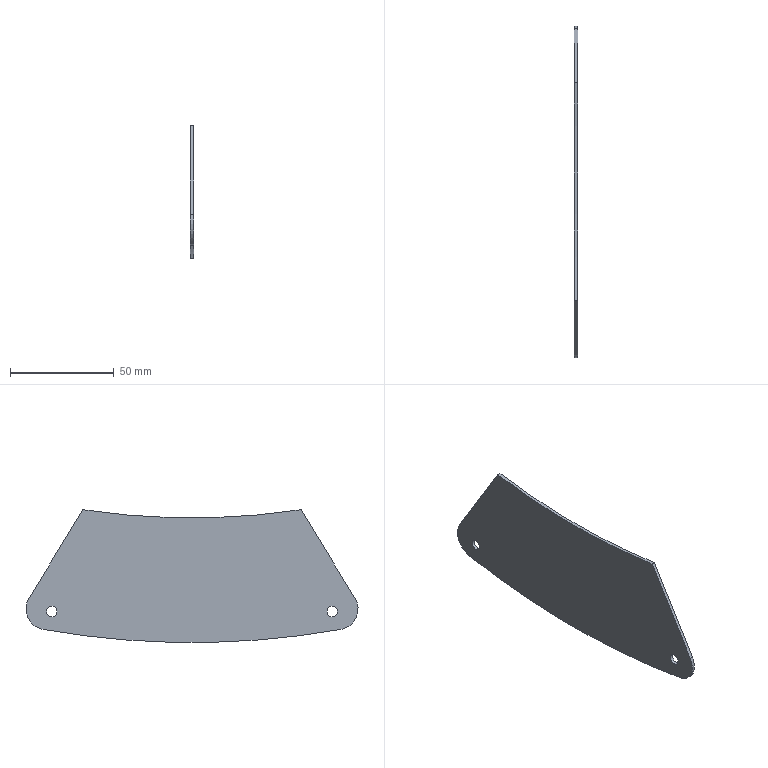Part | STEP file | 1 solid | 10 faces | box 1.5 x 159.863 x 63.96 mm | volume 12341 mm3 | cylinder 6 | plane 4 | commonest cylinder face diameters 5 x2 20 x2 700 x1 820 x1
STEP:
#1=CARTESIAN_POINT('',(0.,0.,0.));
#2=DIRECTION('',(0.,0.,1.));
#3=DIRECTION('',(1.,0.,0.));
#4=AXIS2_PLACEMENT_3D('',#1,#2,#3);
#5=CARTESIAN_POINT('',(25.,-67.5,-397.5));
#6=VERTEX_POINT('',#5);
#7=CARTESIAN_POINT('',(25.,-67.5,-395.));
#8=DIRECTION('',(-1.,0.,0.));
#9=DIRECTION('',(0.,0.,-1.));
#10=AXIS2_PLACEMENT_3D('',#7,#8,#9);
#11=CIRCLE('',#10,2.5);
#12=CARTESIAN_POINT('',(25.,0.,0.));
#13=DIRECTION('',(1.,0.,0.));
#14=DIRECTION('',(0.,0.,-1.));
#15=AXIS2_PLACEMENT_3D('',#12,#13,#14);
#16=PLANE('',#15);
#17=CARTESIAN_POINT('',(397.5,-67.5));
#18=CARTESIAN_POINT('',(397.5,-71.83));
#19=CARTESIAN_POINT('',(393.75,-69.665));
#20=CARTESIAN_POINT('',(390.,-67.5));
#21=CARTESIAN_POINT('',(393.75,-65.335));
#22=CARTESIAN_POINT('',(397.5,-63.17));
#23=CARTESIAN_POINT('',(397.5,-67.5));
#24=(BOUNDED_CURVE()B_SPLINE_CURVE(2,(#17,#18,#19,#20,#21,#22,#23),.UNSPECIFIED.,.T.,.F.)B_SPLINE_CURVE_WITH_KNOTS((1,2,2,2,2,1),(-2.094,0.,2.094,4.189,6.283,8.378),.UNSPECIFIED.)CURVE()GEOMETRIC_REPRESENTATION_ITEM()RATIONAL_B_SPLINE_CURVE((1.,0.5,1.,0.5,1.,0.5,1.))REPRESENTATION_ITEM(''));
#25=(GEOMETRIC_REPRESENTATION_CONTEXT(2)PARAMETRIC_REPRESENTATION_CONTEXT()REPRESENTATION_CONTEXT('',''));
#26=DEFINITIONAL_REPRESENTATION('',(#24),#25);
#27=PCURVE('',#16,#26);
#28=CARTESIAN_POINT('',(26.5,-67.5,-395.));
#29=DIRECTION('',(1.,0.,0.));
#30=DIRECTION('',(0.,0.,-1.));
#31=AXIS2_PLACEMENT_3D('',#28,#29,#30);
#32=CYLINDRICAL_SURFACE('',#31,2.5);
#33=CARTESIAN_POINT('',(6.283,-1.5));
#34=DIRECTION('',(-1.,0.));
#35=VECTOR('',#34,1.);
#36=LINE('',#33,#35);
#37=(GEOMETRIC_REPRESENTATION_CONTEXT(2)PARAMETRIC_REPRESENTATION_CONTEXT()REPRESENTATION_CONTEXT('',''));
#38=DEFINITIONAL_REPRESENTATION('',(#36),#37);
#39=PCURVE('',#32,#38);
#40=SURFACE_CURVE('',#11,(#27,#39),.PCURVE_S1.);
#41=EDGE_CURVE('',#6,#6,#40,.T.);
#42=ORIENTED_EDGE('',*,*,#41,.F.);
#43=EDGE_LOOP('',(#42));
#44=FACE_BOUND('',#43,.T.);
#45=CARTESIAN_POINT('',(25.,67.5,-397.5));
#46=VERTEX_POINT('',#45);
#47=CARTESIAN_POINT('',(25.,67.5,-395.));
#48=DIRECTION('',(-1.,0.,0.));
#49=DIRECTION('',(0.,0.,-1.));
#50=AXIS2_PLACEMENT_3D('',#47,#48,#49);
#51=CIRCLE('',#50,2.5);
#52=CARTESIAN_POINT('',(397.5,67.5));
#53=CARTESIAN_POINT('',(397.5,63.17));
#54=CARTESIAN_POINT('',(393.75,65.335));
#55=CARTESIAN_POINT('',(390.,67.5));
#56=CARTESIAN_POINT('',(393.75,69.665));
#57=CARTESIAN_POINT('',(397.5,71.83));
#58=CARTESIAN_POINT('',(397.5,67.5));
#59=(BOUNDED_CURVE()B_SPLINE_CURVE(2,(#52,#53,#54,#55,#56,#57,#58),.UNSPECIFIED.,.T.,.F.)B_SPLINE_CURVE_WITH_KNOTS((1,2,2,2,2,1),(-2.094,0.,2.094,4.189,6.283,8.378),.UNSPECIFIED.)CURVE()GEOMETRIC_REPRESENTATION_ITEM()RATIONAL_B_SPLINE_CURVE((1.,0.5,1.,0.5,1.,0.5,1.))REPRESENTATION_ITEM(''));
#60=(GEOMETRIC_REPRESENTATION_CONTEXT(2)PARAMETRIC_REPRESENTATION_CONTEXT()REPRESENTATION_CONTEXT('',''));
#61=DEFINITIONAL_REPRESENTATION('',(#59),#60);
#62=PCURVE('',#16,#61);
#63=CARTESIAN_POINT('',(26.5,67.5,-395.));
#64=DIRECTION('',(1.,0.,0.));
#65=DIRECTION('',(0.,0.,-1.));
#66=AXIS2_PLACEMENT_3D('',#63,#64,#65);
#67=CYLINDRICAL_SURFACE('',#66,2.5);
#68=CARTESIAN_POINT('',(6.283,-1.5));
#69=DIRECTION('',(-1.,0.));
#70=VECTOR('',#69,1.);
#71=LINE('',#68,#70);
#72=(GEOMETRIC_REPRESENTATION_CONTEXT(2)PARAMETRIC_REPRESENTATION_CONTEXT()REPRESENTATION_CONTEXT('',''));
#73=DEFINITIONAL_REPRESENTATION('',(#71),#72);
#74=PCURVE('',#67,#73);
#75=SURFACE_CURVE('',#51,(#62,#74),.PCURVE_S1.);
#76=EDGE_CURVE('',#46,#46,#75,.T.);
#77=ORIENTED_EDGE('',*,*,#76,.F.);
#78=EDGE_LOOP('',(#77));
#79=FACE_BOUND('',#78,.T.);
#80=CARTESIAN_POINT('',(25.,-78.469,-388.634));
#81=VERTEX_POINT('',#80);
#82=CARTESIAN_POINT('',(25.,-71.68,-403.686));
#83=VERTEX_POINT('',#82);
#84=CARTESIAN_POINT('',(25.,-69.931,-393.84));
#85=DIRECTION('',(1.,0.,0.));
#86=DIRECTION('',(0.,0.,-1.));
#87=AXIS2_PLACEMENT_3D('',#84,#85,#86);
#88=CIRCLE('',#87,10.);
#89=CARTESIAN_POINT('',(393.84,-69.931));
#90=DIRECTION('',(1.,0.));
#91=AXIS2_PLACEMENT_2D('',#89,#90);
#92=CIRCLE('',#91,10.);
#93=(GEOMETRIC_REPRESENTATION_CONTEXT(2)PARAMETRIC_REPRESENTATION_CONTEXT()REPRESENTATION_CONTEXT('',''));
#94=DEFINITIONAL_REPRESENTATION('',(#92),#93);
#95=PCURVE('',#16,#94);
#96=CARTESIAN_POINT('',(26.5,-69.931,-393.84));
#97=DIRECTION('',(1.,0.,0.));
#98=DIRECTION('',(0.,0.,-1.));
#99=AXIS2_PLACEMENT_3D('',#96,#97,#98);
#100=CYLINDRICAL_SURFACE('',#99,10.);
#101=CARTESIAN_POINT('',(0.,-1.5));
#102=DIRECTION('',(1.,0.));
#103=VECTOR('',#102,1.);
#104=LINE('',#101,#103);
#105=(GEOMETRIC_REPRESENTATION_CONTEXT(2)PARAMETRIC_REPRESENTATION_CONTEXT()REPRESENTATION_CONTEXT('',''));
#106=DEFINITIONAL_REPRESENTATION('',(#104),#105);
#107=PCURVE('',#100,#106);
#108=SURFACE_CURVE('',#88,(#95,#107),.PCURVE_S1.);
#109=EDGE_CURVE('',#81,#83,#108,.T.);
#110=ORIENTED_EDGE('',*,*,#109,.F.);
#111=CARTESIAN_POINT('',(25.,-52.5,-346.04));
#112=VERTEX_POINT('',#111);
#113=CARTESIAN_POINT('',(25.,-52.5,-346.04));
#114=DIRECTION('',(0.,-0.5206,-0.8538));
#115=VECTOR('',#114,1.);
#116=LINE('',#113,#115);
#117=CARTESIAN_POINT('',(346.04,-52.5));
#118=DIRECTION('',(0.8538,-0.5206));
#119=VECTOR('',#118,1.);
#120=LINE('',#117,#119);
#121=(GEOMETRIC_REPRESENTATION_CONTEXT(2)PARAMETRIC_REPRESENTATION_CONTEXT()REPRESENTATION_CONTEXT('',''));
#122=DEFINITIONAL_REPRESENTATION('',(#120),#121);
#123=PCURVE('',#16,#122);
#124=CARTESIAN_POINT('',(26.5,-52.5,-346.04));
#125=DIRECTION('',(0.,-0.8538,0.5206));
#126=DIRECTION('',(0.,-0.5206,-0.8538));
#127=AXIS2_PLACEMENT_3D('',#124,#125,#126);
#128=PLANE('',#127);
#129=CARTESIAN_POINT('',(0.,-1.5));
#130=DIRECTION('',(1.,0.));
#131=VECTOR('',#130,1.);
#132=LINE('',#129,#131);
#133=(GEOMETRIC_REPRESENTATION_CONTEXT(2)PARAMETRIC_REPRESENTATION_CONTEXT()REPRESENTATION_CONTEXT('',''));
#134=DEFINITIONAL_REPRESENTATION('',(#132),#133);
#135=PCURVE('',#128,#134);
#136=SURFACE_CURVE('',#116,(#123,#135),.PCURVE_S1.);
#137=EDGE_CURVE('',#112,#81,#136,.T.);
#138=ORIENTED_EDGE('',*,*,#137,.F.);
#139=CARTESIAN_POINT('',(25.,52.5,-346.04));
#140=VERTEX_POINT('',#139);
#141=CARTESIAN_POINT('',(25.,0.,0.));
#142=DIRECTION('',(-1.,0.,0.));
#143=DIRECTION('',(0.,0.,-1.));
#144=AXIS2_PLACEMENT_3D('',#141,#142,#143);
#145=CIRCLE('',#144,350.);
#146=CARTESIAN_POINT('',(350.,0.));
#147=CARTESIAN_POINT('',(350.,-606.218));
#148=CARTESIAN_POINT('',(-175.,-303.109));
#149=CARTESIAN_POINT('',(-700.,0.));
#150=CARTESIAN_POINT('',(-175.,303.109));
#151=CARTESIAN_POINT('',(350.,606.218));
#152=CARTESIAN_POINT('',(350.,0.));
#153=(BOUNDED_CURVE()B_SPLINE_CURVE(2,(#146,#147,#148,#149,#150,#151,#152),.UNSPECIFIED.,.T.,.F.)B_SPLINE_CURVE_WITH_KNOTS((1,2,2,2,2,1),(-2.094,0.,2.094,4.189,6.283,8.378),.UNSPECIFIED.)CURVE()GEOMETRIC_REPRESENTATION_ITEM()RATIONAL_B_SPLINE_CURVE((1.,0.5,1.,0.5,1.,0.5,1.))REPRESENTATION_ITEM(''));
#154=(GEOMETRIC_REPRESENTATION_CONTEXT(2)PARAMETRIC_REPRESENTATION_CONTEXT()REPRESENTATION_CONTEXT('',''));
#155=DEFINITIONAL_REPRESENTATION('',(#153),#154);
#156=PCURVE('',#16,#155);
#157=CARTESIAN_POINT('',(26.5,0.,0.));
#158=DIRECTION('',(1.,0.,0.));
#159=DIRECTION('',(0.,0.,-1.));
#160=AXIS2_PLACEMENT_3D('',#157,#158,#159);
#161=CYLINDRICAL_SURFACE('',#160,350.);
#162=CARTESIAN_POINT('',(12.566,-1.5));
#163=DIRECTION('',(-1.,0.));
#164=VECTOR('',#163,1.);
#165=LINE('',#162,#164);
#166=(GEOMETRIC_REPRESENTATION_CONTEXT(2)PARAMETRIC_REPRESENTATION_CONTEXT()REPRESENTATION_CONTEXT('',''));
#167=DEFINITIONAL_REPRESENTATION('',(#165),#166);
#168=PCURVE('',#161,#167);
#169=SURFACE_CURVE('',#145,(#156,#168),.PCURVE_S1.);
#170=EDGE_CURVE('',#140,#112,#169,.T.);
#171=ORIENTED_EDGE('',*,*,#170,.F.);
#172=CARTESIAN_POINT('',(25.,78.469,-388.634));
#173=VERTEX_POINT('',#172);
#174=CARTESIAN_POINT('',(25.,78.469,-388.634));
#175=DIRECTION('',(0.,-0.5206,0.8538));
#176=VECTOR('',#175,1.);
#177=LINE('',#174,#176);
#178=CARTESIAN_POINT('',(388.634,78.469));
#179=DIRECTION('',(-0.8538,-0.5206));
#180=VECTOR('',#179,1.);
#181=LINE('',#178,#180);
#182=(GEOMETRIC_REPRESENTATION_CONTEXT(2)PARAMETRIC_REPRESENTATION_CONTEXT()REPRESENTATION_CONTEXT('',''));
#183=DEFINITIONAL_REPRESENTATION('',(#181),#182);
#184=PCURVE('',#16,#183);
#185=CARTESIAN_POINT('',(26.5,52.5,-346.04));
#186=DIRECTION('',(0.,0.8538,0.5206));
#187=DIRECTION('',(0.,-0.5206,0.8538));
#188=AXIS2_PLACEMENT_3D('',#185,#186,#187);
#189=PLANE('',#188);
#190=CARTESIAN_POINT('',(-49.886,-1.5));
#191=DIRECTION('',(1.,0.));
#192=VECTOR('',#191,1.);
#193=LINE('',#190,#192);
#194=(GEOMETRIC_REPRESENTATION_CONTEXT(2)PARAMETRIC_REPRESENTATION_CONTEXT()REPRESENTATION_CONTEXT('',''));
#195=DEFINITIONAL_REPRESENTATION('',(#193),#194);
#196=PCURVE('',#189,#195);
#197=SURFACE_CURVE('',#177,(#184,#196),.PCURVE_S1.);
#198=EDGE_CURVE('',#173,#140,#197,.T.);
#199=ORIENTED_EDGE('',*,*,#198,.F.);
#200=CARTESIAN_POINT('',(25.,71.68,-403.686));
#201=VERTEX_POINT('',#200);
#202=CARTESIAN_POINT('',(25.,69.931,-393.84));
#203=DIRECTION('',(1.,0.,0.));
#204=DIRECTION('',(0.,0.,-1.));
#205=AXIS2_PLACEMENT_3D('',#202,#203,#204);
#206=CIRCLE('',#205,10.);
#207=CARTESIAN_POINT('',(393.84,69.931));
#208=DIRECTION('',(1.,0.));
#209=AXIS2_PLACEMENT_2D('',#207,#208);
#210=CIRCLE('',#209,10.);
#211=(GEOMETRIC_REPRESENTATION_CONTEXT(2)PARAMETRIC_REPRESENTATION_CONTEXT()REPRESENTATION_CONTEXT('',''));
#212=DEFINITIONAL_REPRESENTATION('',(#210),#211);
#213=PCURVE('',#16,#212);
#214=CARTESIAN_POINT('',(26.5,69.931,-393.84));
#215=DIRECTION('',(1.,0.,0.));
#216=DIRECTION('',(0.,0.,-1.));
#217=AXIS2_PLACEMENT_3D('',#214,#215,#216);
#218=CYLINDRICAL_SURFACE('',#217,10.);
#219=CARTESIAN_POINT('',(0.,-1.5));
#220=DIRECTION('',(1.,0.));
#221=VECTOR('',#220,1.);
#222=LINE('',#219,#221);
#223=(GEOMETRIC_REPRESENTATION_CONTEXT(2)PARAMETRIC_REPRESENTATION_CONTEXT()REPRESENTATION_CONTEXT('',''));
#224=DEFINITIONAL_REPRESENTATION('',(#222),#223);
#225=PCURVE('',#218,#224);
#226=SURFACE_CURVE('',#206,(#213,#225),.PCURVE_S1.);
#227=EDGE_CURVE('',#201,#173,#226,.T.);
#228=ORIENTED_EDGE('',*,*,#227,.F.);
#229=CARTESIAN_POINT('',(25.,0.,0.));
#230=DIRECTION('',(1.,0.,0.));
#231=DIRECTION('',(0.,0.,-1.));
#232=AXIS2_PLACEMENT_3D('',#229,#230,#231);
#233=CIRCLE('',#232,410.);
#234=CARTESIAN_POINT('',(0.,0.));
#235=DIRECTION('',(1.,0.));
#236=AXIS2_PLACEMENT_2D('',#234,#235);
#237=CIRCLE('',#236,410.);
#238=(GEOMETRIC_REPRESENTATION_CONTEXT(2)PARAMETRIC_REPRESENTATION_CONTEXT()REPRESENTATION_CONTEXT('',''));
#239=DEFINITIONAL_REPRESENTATION('',(#237),#238);
#240=PCURVE('',#16,#239);
#241=CARTESIAN_POINT('',(26.5,0.,0.));
#242=DIRECTION('',(1.,0.,0.));
#243=DIRECTION('',(0.,0.,-1.));
#244=AXIS2_PLACEMENT_3D('',#241,#242,#243);
#245=CYLINDRICAL_SURFACE('',#244,410.);
#246=CARTESIAN_POINT('',(-6.283,-1.5));
#247=DIRECTION('',(1.,0.));
#248=VECTOR('',#247,1.);
#249=LINE('',#246,#248);
#250=(GEOMETRIC_REPRESENTATION_CONTEXT(2)PARAMETRIC_REPRESENTATION_CONTEXT()REPRESENTATION_CONTEXT('',''));
#251=DEFINITIONAL_REPRESENTATION('',(#249),#250);
#252=PCURVE('',#245,#251);
#253=SURFACE_CURVE('',#233,(#240,#252),.PCURVE_S1.);
#254=EDGE_CURVE('',#83,#201,#253,.T.);
#255=ORIENTED_EDGE('',*,*,#254,.F.);
#256=EDGE_LOOP('',(#110,#138,#171,#199,#228,#255));
#257=FACE_BOUND('',#256,.T.);
#258=ADVANCED_FACE('',(#44,#79,#257),#16,.F.);
#259=ORIENTED_EDGE('',*,*,#41,.F.);
#260=CARTESIAN_POINT('',(26.5,-67.5,-397.5));
#261=VERTEX_POINT('',#260);
#262=CARTESIAN_POINT('',(25.,-67.5,-397.5));
#263=CARTESIAN_POINT('',(26.5,-67.5,-397.5));
#264=B_SPLINE_CURVE_WITH_KNOTS('',1,(#262,#263),.UNSPECIFIED.,.F.,.F.,(2,2),(-1.5,0.),.PIECEWISE_BEZIER_KNOTS.);
#265=CARTESIAN_POINT('',(6.283,0.));
#266=DIRECTION('',(0.,1.));
#267=VECTOR('',#266,1.);
#268=LINE('',#265,#267);
#269=(GEOMETRIC_REPRESENTATION_CONTEXT(2)PARAMETRIC_REPRESENTATION_CONTEXT()REPRESENTATION_CONTEXT('',''));
#270=DEFINITIONAL_REPRESENTATION('',(#268),#269);
#271=PCURVE('',#32,#270);
#272=CARTESIAN_POINT('',(0.,0.));
#273=DIRECTION('',(0.,1.));
#274=VECTOR('',#273,1.);
#275=LINE('',#272,#274);
#276=(GEOMETRIC_REPRESENTATION_CONTEXT(2)PARAMETRIC_REPRESENTATION_CONTEXT()REPRESENTATION_CONTEXT('',''));
#277=DEFINITIONAL_REPRESENTATION('',(#275),#276);
#278=PCURVE('',#32,#277);
#279=SEAM_CURVE('',#264,(#271,#278),.PCURVE_S1.);
#280=EDGE_CURVE('',#6,#261,#279,.T.);
#281=ORIENTED_EDGE('',*,*,#280,.T.);
#282=CARTESIAN_POINT('',(26.5,-67.5,-395.));
#283=DIRECTION('',(-1.,0.,0.));
#284=DIRECTION('',(0.,0.,-1.));
#285=AXIS2_PLACEMENT_3D('',#282,#283,#284);
#286=CIRCLE('',#285,2.5);
#287=CARTESIAN_POINT('',(6.283,0.));
#288=DIRECTION('',(-1.,0.));
#289=VECTOR('',#288,1.);
#290=LINE('',#287,#289);
#291=(GEOMETRIC_REPRESENTATION_CONTEXT(2)PARAMETRIC_REPRESENTATION_CONTEXT()REPRESENTATION_CONTEXT('',''));
#292=DEFINITIONAL_REPRESENTATION('',(#290),#291);
#293=PCURVE('',#32,#292);
#294=CARTESIAN_POINT('',(26.5,0.,0.));
#295=DIRECTION('',(1.,0.,0.));
#296=DIRECTION('',(0.,0.,-1.));
#297=AXIS2_PLACEMENT_3D('',#294,#295,#296);
#298=PLANE('',#297);
#299=CARTESIAN_POINT('',(397.5,-67.5));
#300=CARTESIAN_POINT('',(397.5,-71.83));
#301=CARTESIAN_POINT('',(393.75,-69.665));
#302=CARTESIAN_POINT('',(390.,-67.5));
#303=CARTESIAN_POINT('',(393.75,-65.335));
#304=CARTESIAN_POINT('',(397.5,-63.17));
#305=CARTESIAN_POINT('',(397.5,-67.5));
#306=(BOUNDED_CURVE()B_SPLINE_CURVE(2,(#299,#300,#301,#302,#303,#304,#305),.UNSPECIFIED.,.T.,.F.)B_SPLINE_CURVE_WITH_KNOTS((1,2,2,2,2,1),(-2.094,0.,2.094,4.189,6.283,8.378),.UNSPECIFIED.)CURVE()GEOMETRIC_REPRESENTATION_ITEM()RATIONAL_B_SPLINE_CURVE((1.,0.5,1.,0.5,1.,0.5,1.))REPRESENTATION_ITEM(''));
#307=(GEOMETRIC_REPRESENTATION_CONTEXT(2)PARAMETRIC_REPRESENTATION_CONTEXT()REPRESENTATION_CONTEXT('',''));
#308=DEFINITIONAL_REPRESENTATION('',(#306),#307);
#309=PCURVE('',#298,#308);
#310=SURFACE_CURVE('',#286,(#293,#309),.PCURVE_S1.);
#311=EDGE_CURVE('',#261,#261,#310,.T.);
#312=ORIENTED_EDGE('',*,*,#311,.T.);
#313=ORIENTED_EDGE('',*,*,#280,.F.);
#314=EDGE_LOOP('',(#259,#281,#312,#313));
#315=FACE_BOUND('',#314,.F.);
#316=ADVANCED_FACE('',(#315),#32,.F.);
#317=ORIENTED_EDGE('',*,*,#76,.F.);
#318=CARTESIAN_POINT('',(26.5,67.5,-397.5));
#319=VERTEX_POINT('',#318);
#320=CARTESIAN_POINT('',(25.,67.5,-397.5));
#321=CARTESIAN_POINT('',(26.5,67.5,-397.5));
#322=B_SPLINE_CURVE_WITH_KNOTS('',1,(#320,#321),.UNSPECIFIED.,.F.,.F.,(2,2),(-1.5,0.),.PIECEWISE_BEZIER_KNOTS.);
#323=CARTESIAN_POINT('',(6.283,0.));
#324=DIRECTION('',(0.,1.));
#325=VECTOR('',#324,1.);
#326=LINE('',#323,#325);
#327=(GEOMETRIC_REPRESENTATION_CONTEXT(2)PARAMETRIC_REPRESENTATION_CONTEXT()REPRESENTATION_CONTEXT('',''));
#328=DEFINITIONAL_REPRESENTATION('',(#326),#327);
#329=PCURVE('',#67,#328);
#330=CARTESIAN_POINT('',(0.,0.));
#331=DIRECTION('',(0.,1.));
#332=VECTOR('',#331,1.);
#333=LINE('',#330,#332);
#334=(GEOMETRIC_REPRESENTATION_CONTEXT(2)PARAMETRIC_REPRESENTATION_CONTEXT()REPRESENTATION_CONTEXT('',''));
#335=DEFINITIONAL_REPRESENTATION('',(#333),#334);
#336=PCURVE('',#67,#335);
#337=SEAM_CURVE('',#322,(#329,#336),.PCURVE_S1.);
#338=EDGE_CURVE('',#46,#319,#337,.T.);
#339=ORIENTED_EDGE('',*,*,#338,.T.);
#340=CARTESIAN_POINT('',(26.5,67.5,-395.));
#341=DIRECTION('',(-1.,0.,0.));
#342=DIRECTION('',(0.,0.,-1.));
#343=AXIS2_PLACEMENT_3D('',#340,#341,#342);
#344=CIRCLE('',#343,2.5);
#345=CARTESIAN_POINT('',(6.283,0.));
#346=DIRECTION('',(-1.,0.));
#347=VECTOR('',#346,1.);
#348=LINE('',#345,#347);
#349=(GEOMETRIC_REPRESENTATION_CONTEXT(2)PARAMETRIC_REPRESENTATION_CONTEXT()REPRESENTATION_CONTEXT('',''));
#350=DEFINITIONAL_REPRESENTATION('',(#348),#349);
#351=PCURVE('',#67,#350);
#352=CARTESIAN_POINT('',(397.5,67.5));
#353=CARTESIAN_POINT('',(397.5,63.17));
#354=CARTESIAN_POINT('',(393.75,65.335));
#355=CARTESIAN_POINT('',(390.,67.5));
#356=CARTESIAN_POINT('',(393.75,69.665));
#357=CARTESIAN_POINT('',(397.5,71.83));
#358=CARTESIAN_POINT('',(397.5,67.5));
#359=(BOUNDED_CURVE()B_SPLINE_CURVE(2,(#352,#353,#354,#355,#356,#357,#358),.UNSPECIFIED.,.T.,.F.)B_SPLINE_CURVE_WITH_KNOTS((1,2,2,2,2,1),(-2.094,0.,2.094,4.189,6.283,8.378),.UNSPECIFIED.)CURVE()GEOMETRIC_REPRESENTATION_ITEM()RATIONAL_B_SPLINE_CURVE((1.,0.5,1.,0.5,1.,0.5,1.))REPRESENTATION_ITEM(''));
#360=(GEOMETRIC_REPRESENTATION_CONTEXT(2)PARAMETRIC_REPRESENTATION_CONTEXT()REPRESENTATION_CONTEXT('',''));
#361=DEFINITIONAL_REPRESENTATION('',(#359),#360);
#362=PCURVE('',#298,#361);
#363=SURFACE_CURVE('',#344,(#351,#362),.PCURVE_S1.);
#364=EDGE_CURVE('',#319,#319,#363,.T.);
#365=ORIENTED_EDGE('',*,*,#364,.T.);
#366=ORIENTED_EDGE('',*,*,#338,.F.);
#367=EDGE_LOOP('',(#317,#339,#365,#366));
#368=FACE_BOUND('',#367,.F.);
#369=ADVANCED_FACE('',(#368),#67,.F.);
#370=CARTESIAN_POINT('',(26.5,71.68,-403.686));
#371=VERTEX_POINT('',#370);
#372=CARTESIAN_POINT('',(26.5,-71.68,-403.686));
#373=VERTEX_POINT('',#372);
#374=CARTESIAN_POINT('',(26.5,0.,0.));
#375=DIRECTION('',(-1.,0.,0.));
#376=DIRECTION('',(0.,0.,-1.));
#377=AXIS2_PLACEMENT_3D('',#374,#375,#376);
#378=CIRCLE('',#377,410.);
#379=CARTESIAN_POINT('',(6.283,0.));
#380=DIRECTION('',(-1.,0.));
#381=VECTOR('',#380,1.);
#382=LINE('',#379,#381);
#383=(GEOMETRIC_REPRESENTATION_CONTEXT(2)PARAMETRIC_REPRESENTATION_CONTEXT()REPRESENTATION_CONTEXT('',''));
#384=DEFINITIONAL_REPRESENTATION('',(#382),#383);
#385=PCURVE('',#245,#384);
#386=CARTESIAN_POINT('',(410.,0.));
#387=CARTESIAN_POINT('',(410.,-710.141));
#388=CARTESIAN_POINT('',(-205.,-355.07));
#389=CARTESIAN_POINT('',(-820.,0.));
#390=CARTESIAN_POINT('',(-205.,355.07));
#391=CARTESIAN_POINT('',(410.,710.141));
#392=CARTESIAN_POINT('',(410.,0.));
#393=(BOUNDED_CURVE()B_SPLINE_CURVE(2,(#386,#387,#388,#389,#390,#391,#392),.UNSPECIFIED.,.T.,.F.)B_SPLINE_CURVE_WITH_KNOTS((1,2,2,2,2,1),(-2.094,0.,2.094,4.189,6.283,8.378),.UNSPECIFIED.)CURVE()GEOMETRIC_REPRESENTATION_ITEM()RATIONAL_B_SPLINE_CURVE((1.,0.5,1.,0.5,1.,0.5,1.))REPRESENTATION_ITEM(''));
#394=(GEOMETRIC_REPRESENTATION_CONTEXT(2)PARAMETRIC_REPRESENTATION_CONTEXT()REPRESENTATION_CONTEXT('',''));
#395=DEFINITIONAL_REPRESENTATION('',(#393),#394);
#396=PCURVE('',#298,#395);
#397=SURFACE_CURVE('',#378,(#385,#396),.PCURVE_S1.);
#398=EDGE_CURVE('',#371,#373,#397,.T.);
#399=ORIENTED_EDGE('',*,*,#398,.T.);
#400=CARTESIAN_POINT('',(26.5,-71.68,-403.686));
#401=DIRECTION('',(-1.,0.,0.));
#402=VECTOR('',#401,1.);
#403=LINE('',#400,#402);
#404=CARTESIAN_POINT('',(-0.1757,0.));
#405=DIRECTION('',(0.,-1.));
#406=VECTOR('',#405,1.);
#407=LINE('',#404,#406);
#408=(GEOMETRIC_REPRESENTATION_CONTEXT(2)PARAMETRIC_REPRESENTATION_CONTEXT()REPRESENTATION_CONTEXT('',''));
#409=DEFINITIONAL_REPRESENTATION('',(#407),#408);
#410=PCURVE('',#245,#409);
#411=CARTESIAN_POINT('',(6.107,0.));
#412=DIRECTION('',(0.,-1.));
#413=VECTOR('',#412,1.);
#414=LINE('',#411,#413);
#415=(GEOMETRIC_REPRESENTATION_CONTEXT(2)PARAMETRIC_REPRESENTATION_CONTEXT()REPRESENTATION_CONTEXT('',''));
#416=DEFINITIONAL_REPRESENTATION('',(#414),#415);
#417=PCURVE('',#100,#416);
#418=SURFACE_CURVE('',#403,(#410,#417),.PCURVE_S1.);
#419=EDGE_CURVE('',#373,#83,#418,.T.);
#420=ORIENTED_EDGE('',*,*,#419,.T.);
#421=ORIENTED_EDGE('',*,*,#254,.T.);
#422=CARTESIAN_POINT('',(26.5,71.68,-403.686));
#423=DIRECTION('',(-1.,0.,0.));
#424=VECTOR('',#423,1.);
#425=LINE('',#422,#424);
#426=CARTESIAN_POINT('',(0.1757,0.));
#427=DIRECTION('',(0.,-1.));
#428=VECTOR('',#427,1.);
#429=LINE('',#426,#428);
#430=(GEOMETRIC_REPRESENTATION_CONTEXT(2)PARAMETRIC_REPRESENTATION_CONTEXT()REPRESENTATION_CONTEXT('',''));
#431=DEFINITIONAL_REPRESENTATION('',(#429),#430);
#432=PCURVE('',#245,#431);
#433=CARTESIAN_POINT('',(0.1757,0.));
#434=DIRECTION('',(0.,-1.));
#435=VECTOR('',#434,1.);
#436=LINE('',#433,#435);
#437=(GEOMETRIC_REPRESENTATION_CONTEXT(2)PARAMETRIC_REPRESENTATION_CONTEXT()REPRESENTATION_CONTEXT('',''));
#438=DEFINITIONAL_REPRESENTATION('',(#436),#437);
#439=PCURVE('',#218,#438);
#440=SURFACE_CURVE('',#425,(#432,#439),.PCURVE_S1.);
#441=EDGE_CURVE('',#371,#201,#440,.T.);
#442=ORIENTED_EDGE('',*,*,#441,.F.);
#443=EDGE_LOOP('',(#399,#420,#421,#442));
#444=FACE_BOUND('',#443,.T.);
#445=ADVANCED_FACE('',(#444),#245,.T.);
#446=ORIENTED_EDGE('',*,*,#419,.F.);
#447=CARTESIAN_POINT('',(26.5,-78.469,-388.634));
#448=VERTEX_POINT('',#447);
#449=CARTESIAN_POINT('',(26.5,-69.931,-393.84));
#450=DIRECTION('',(-1.,0.,0.));
#451=DIRECTION('',(0.,0.,-1.));
#452=AXIS2_PLACEMENT_3D('',#449,#450,#451);
#453=CIRCLE('',#452,10.);
#454=CARTESIAN_POINT('',(6.283,0.));
#455=DIRECTION('',(-1.,0.));
#456=VECTOR('',#455,1.);
#457=LINE('',#454,#456);
#458=(GEOMETRIC_REPRESENTATION_CONTEXT(2)PARAMETRIC_REPRESENTATION_CONTEXT()REPRESENTATION_CONTEXT('',''));
#459=DEFINITIONAL_REPRESENTATION('',(#457),#458);
#460=PCURVE('',#100,#459);
#461=CARTESIAN_POINT('',(403.84,-69.931));
#462=CARTESIAN_POINT('',(403.84,-87.252));
#463=CARTESIAN_POINT('',(388.84,-78.592));
#464=CARTESIAN_POINT('',(373.84,-69.931));
#465=CARTESIAN_POINT('',(388.84,-61.271));
#466=CARTESIAN_POINT('',(403.84,-52.611));
#467=CARTESIAN_POINT('',(403.84,-69.931));
#468=(BOUNDED_CURVE()B_SPLINE_CURVE(2,(#461,#462,#463,#464,#465,#466,#467),.UNSPECIFIED.,.T.,.F.)B_SPLINE_CURVE_WITH_KNOTS((1,2,2,2,2,1),(-2.094,0.,2.094,4.189,6.283,8.378),.UNSPECIFIED.)CURVE()GEOMETRIC_REPRESENTATION_ITEM()RATIONAL_B_SPLINE_CURVE((1.,0.5,1.,0.5,1.,0.5,1.))REPRESENTATION_ITEM(''));
#469=(GEOMETRIC_REPRESENTATION_CONTEXT(2)PARAMETRIC_REPRESENTATION_CONTEXT()REPRESENTATION_CONTEXT('',''));
#470=DEFINITIONAL_REPRESENTATION('',(#468),#469);
#471=PCURVE('',#298,#470);
#472=SURFACE_CURVE('',#453,(#460,#471),.PCURVE_S1.);
#473=EDGE_CURVE('',#373,#448,#472,.T.);
#474=ORIENTED_EDGE('',*,*,#473,.T.);
#475=CARTESIAN_POINT('',(26.5,-78.469,-388.634));
#476=DIRECTION('',(-1.,0.,0.));
#477=VECTOR('',#476,1.);
#478=LINE('',#475,#477);
#479=CARTESIAN_POINT('',(4.165,0.));
#480=DIRECTION('',(0.,-1.));
#481=VECTOR('',#480,1.);
#482=LINE('',#479,#481);
#483=(GEOMETRIC_REPRESENTATION_CONTEXT(2)PARAMETRIC_REPRESENTATION_CONTEXT()REPRESENTATION_CONTEXT('',''));
#484=DEFINITIONAL_REPRESENTATION('',(#482),#483);
#485=PCURVE('',#100,#484);
#486=CARTESIAN_POINT('',(49.886,0.));
#487=DIRECTION('',(0.,-1.));
#488=VECTOR('',#487,1.);
#489=LINE('',#486,#488);
#490=(GEOMETRIC_REPRESENTATION_CONTEXT(2)PARAMETRIC_REPRESENTATION_CONTEXT()REPRESENTATION_CONTEXT('',''));
#491=DEFINITIONAL_REPRESENTATION('',(#489),#490);
#492=PCURVE('',#128,#491);
#493=SURFACE_CURVE('',#478,(#485,#492),.PCURVE_S1.);
#494=EDGE_CURVE('',#448,#81,#493,.T.);
#495=ORIENTED_EDGE('',*,*,#494,.T.);
#496=ORIENTED_EDGE('',*,*,#109,.T.);
#497=EDGE_LOOP('',(#446,#474,#495,#496));
#498=FACE_BOUND('',#497,.T.);
#499=ADVANCED_FACE('',(#498),#100,.T.);
#500=ORIENTED_EDGE('',*,*,#494,.F.);
#501=CARTESIAN_POINT('',(26.5,-52.5,-346.04));
#502=VERTEX_POINT('',#501);
#503=CARTESIAN_POINT('',(26.5,-52.5,-346.04));
#504=DIRECTION('',(0.,0.5206,0.8538));
#505=VECTOR('',#504,1.);
#506=LINE('',#503,#505);
#507=CARTESIAN_POINT('',(0.,0.));
#508=DIRECTION('',(-1.,0.));
#509=VECTOR('',#508,1.);
#510=LINE('',#507,#509);
#511=(GEOMETRIC_REPRESENTATION_CONTEXT(2)PARAMETRIC_REPRESENTATION_CONTEXT()REPRESENTATION_CONTEXT('',''));
#512=DEFINITIONAL_REPRESENTATION('',(#510),#511);
#513=PCURVE('',#128,#512);
#514=CARTESIAN_POINT('',(346.04,-52.5));
#515=DIRECTION('',(-0.8538,0.5206));
#516=VECTOR('',#515,1.);
#517=LINE('',#514,#516);
#518=(GEOMETRIC_REPRESENTATION_CONTEXT(2)PARAMETRIC_REPRESENTATION_CONTEXT()REPRESENTATION_CONTEXT('',''));
#519=DEFINITIONAL_REPRESENTATION('',(#517),#518);
#520=PCURVE('',#298,#519);
#521=SURFACE_CURVE('',#506,(#513,#520),.PCURVE_S1.);
#522=EDGE_CURVE('',#448,#502,#521,.T.);
#523=ORIENTED_EDGE('',*,*,#522,.T.);
#524=CARTESIAN_POINT('',(26.5,-52.5,-346.04));
#525=DIRECTION('',(-1.,0.,0.));
#526=VECTOR('',#525,1.);
#527=LINE('',#524,#526);
#528=CARTESIAN_POINT('',(0.,0.));
#529=DIRECTION('',(0.,-1.));
#530=VECTOR('',#529,1.);
#531=LINE('',#528,#530);
#532=(GEOMETRIC_REPRESENTATION_CONTEXT(2)PARAMETRIC_REPRESENTATION_CONTEXT()REPRESENTATION_CONTEXT('',''));
#533=DEFINITIONAL_REPRESENTATION('',(#531),#532);
#534=PCURVE('',#128,#533);
#535=CARTESIAN_POINT('',(6.133,0.));
#536=DIRECTION('',(0.,-1.));
#537=VECTOR('',#536,1.);
#538=LINE('',#535,#537);
#539=(GEOMETRIC_REPRESENTATION_CONTEXT(2)PARAMETRIC_REPRESENTATION_CONTEXT()REPRESENTATION_CONTEXT('',''));
#540=DEFINITIONAL_REPRESENTATION('',(#538),#539);
#541=PCURVE('',#161,#540);
#542=SURFACE_CURVE('',#527,(#534,#541),.PCURVE_S1.);
#543=EDGE_CURVE('',#502,#112,#542,.T.);
#544=ORIENTED_EDGE('',*,*,#543,.T.);
#545=ORIENTED_EDGE('',*,*,#137,.T.);
#546=EDGE_LOOP('',(#500,#523,#544,#545));
#547=FACE_BOUND('',#546,.T.);
#548=ADVANCED_FACE('',(#547),#128,.T.);
#549=CARTESIAN_POINT('',(26.5,52.5,-346.04));
#550=VERTEX_POINT('',#549);
#551=CARTESIAN_POINT('',(26.5,52.5,-346.04));
#552=DIRECTION('',(1.,0.,0.));
#553=VECTOR('',#552,1.);
#554=LINE('',#551,#553);
#555=CARTESIAN_POINT('',(6.434,0.));
#556=DIRECTION('',(0.,1.));
#557=VECTOR('',#556,1.);
#558=LINE('',#555,#557);
#559=(GEOMETRIC_REPRESENTATION_CONTEXT(2)PARAMETRIC_REPRESENTATION_CONTEXT()REPRESENTATION_CONTEXT('',''));
#560=DEFINITIONAL_REPRESENTATION('',(#558),#559);
#561=PCURVE('',#161,#560);
#562=CARTESIAN_POINT('',(0.,0.));
#563=DIRECTION('',(0.,1.));
#564=VECTOR('',#563,1.);
#565=LINE('',#562,#564);
#566=(GEOMETRIC_REPRESENTATION_CONTEXT(2)PARAMETRIC_REPRESENTATION_CONTEXT()REPRESENTATION_CONTEXT('',''));
#567=DEFINITIONAL_REPRESENTATION('',(#565),#566);
#568=PCURVE('',#189,#567);
#569=SURFACE_CURVE('',#554,(#561,#568),.PCURVE_S1.);
#570=EDGE_CURVE('',#140,#550,#569,.T.);
#571=ORIENTED_EDGE('',*,*,#570,.T.);
#572=CARTESIAN_POINT('',(26.5,0.,0.));
#573=DIRECTION('',(-1.,0.,0.));
#574=DIRECTION('',(0.,0.,-1.));
#575=AXIS2_PLACEMENT_3D('',#572,#573,#574);
#576=CIRCLE('',#575,350.);
#577=CARTESIAN_POINT('',(12.566,0.));
#578=DIRECTION('',(-1.,0.));
#579=VECTOR('',#578,1.);
#580=LINE('',#577,#579);
#581=(GEOMETRIC_REPRESENTATION_CONTEXT(2)PARAMETRIC_REPRESENTATION_CONTEXT()REPRESENTATION_CONTEXT('',''));
#582=DEFINITIONAL_REPRESENTATION('',(#580),#581);
#583=PCURVE('',#161,#582);
#584=CARTESIAN_POINT('',(350.,0.));
#585=CARTESIAN_POINT('',(350.,-606.218));
#586=CARTESIAN_POINT('',(-175.,-303.109));
#587=CARTESIAN_POINT('',(-700.,0.));
#588=CARTESIAN_POINT('',(-175.,303.109));
#589=CARTESIAN_POINT('',(350.,606.218));
#590=CARTESIAN_POINT('',(350.,0.));
#591=(BOUNDED_CURVE()B_SPLINE_CURVE(2,(#584,#585,#586,#587,#588,#589,#590),.UNSPECIFIED.,.T.,.F.)B_SPLINE_CURVE_WITH_KNOTS((1,2,2,2,2,1),(-2.094,0.,2.094,4.189,6.283,8.378),.UNSPECIFIED.)CURVE()GEOMETRIC_REPRESENTATION_ITEM()RATIONAL_B_SPLINE_CURVE((1.,0.5,1.,0.5,1.,0.5,1.))REPRESENTATION_ITEM(''));
#592=(GEOMETRIC_REPRESENTATION_CONTEXT(2)PARAMETRIC_REPRESENTATION_CONTEXT()REPRESENTATION_CONTEXT('',''));
#593=DEFINITIONAL_REPRESENTATION('',(#591),#592);
#594=PCURVE('',#298,#593);
#595=SURFACE_CURVE('',#576,(#583,#594),.PCURVE_S1.);
#596=EDGE_CURVE('',#550,#502,#595,.T.);
#597=ORIENTED_EDGE('',*,*,#596,.T.);
#598=ORIENTED_EDGE('',*,*,#543,.T.);
#599=ORIENTED_EDGE('',*,*,#170,.F.);
#600=EDGE_LOOP('',(#571,#597,#598,#599));
#601=FACE_BOUND('',#600,.F.);
#602=ADVANCED_FACE('',(#601),#161,.F.);
#603=ORIENTED_EDGE('',*,*,#570,.T.);
#604=CARTESIAN_POINT('',(26.5,78.469,-388.634));
#605=VERTEX_POINT('',#604);
#606=CARTESIAN_POINT('',(26.5,52.5,-346.04));
#607=DIRECTION('',(0.,0.5206,-0.8538));
#608=VECTOR('',#607,1.);
#609=LINE('',#606,#608);
#610=CARTESIAN_POINT('',(0.,0.));
#611=DIRECTION('',(-1.,0.));
#612=VECTOR('',#611,1.);
#613=LINE('',#610,#612);
#614=(GEOMETRIC_REPRESENTATION_CONTEXT(2)PARAMETRIC_REPRESENTATION_CONTEXT()REPRESENTATION_CONTEXT('',''));
#615=DEFINITIONAL_REPRESENTATION('',(#613),#614);
#616=PCURVE('',#189,#615);
#617=CARTESIAN_POINT('',(346.04,52.5));
#618=DIRECTION('',(0.8538,0.5206));
#619=VECTOR('',#618,1.);
#620=LINE('',#617,#619);
#621=(GEOMETRIC_REPRESENTATION_CONTEXT(2)PARAMETRIC_REPRESENTATION_CONTEXT()REPRESENTATION_CONTEXT('',''));
#622=DEFINITIONAL_REPRESENTATION('',(#620),#621);
#623=PCURVE('',#298,#622);
#624=SURFACE_CURVE('',#609,(#616,#623),.PCURVE_S1.);
#625=EDGE_CURVE('',#550,#605,#624,.T.);
#626=ORIENTED_EDGE('',*,*,#625,.T.);
#627=CARTESIAN_POINT('',(26.5,78.469,-388.634));
#628=DIRECTION('',(-1.,0.,0.));
#629=VECTOR('',#628,1.);
#630=LINE('',#627,#629);
#631=CARTESIAN_POINT('',(-49.886,0.));
#632=DIRECTION('',(0.,-1.));
#633=VECTOR('',#632,1.);
#634=LINE('',#631,#633);
#635=(GEOMETRIC_REPRESENTATION_CONTEXT(2)PARAMETRIC_REPRESENTATION_CONTEXT()REPRESENTATION_CONTEXT('',''));
#636=DEFINITIONAL_REPRESENTATION('',(#634),#635);
#637=PCURVE('',#189,#636);
#638=CARTESIAN_POINT('',(2.118,0.));
#639=DIRECTION('',(0.,-1.));
#640=VECTOR('',#639,1.);
#641=LINE('',#638,#640);
#642=(GEOMETRIC_REPRESENTATION_CONTEXT(2)PARAMETRIC_REPRESENTATION_CONTEXT()REPRESENTATION_CONTEXT('',''));
#643=DEFINITIONAL_REPRESENTATION('',(#641),#642);
#644=PCURVE('',#218,#643);
#645=SURFACE_CURVE('',#630,(#637,#644),.PCURVE_S1.);
#646=EDGE_CURVE('',#605,#173,#645,.T.);
#647=ORIENTED_EDGE('',*,*,#646,.T.);
#648=ORIENTED_EDGE('',*,*,#198,.T.);
#649=EDGE_LOOP('',(#603,#626,#647,#648));
#650=FACE_BOUND('',#649,.T.);
#651=ADVANCED_FACE('',(#650),#189,.T.);
#652=CARTESIAN_POINT('',(26.5,69.931,-393.84));
#653=DIRECTION('',(-1.,0.,0.));
#654=DIRECTION('',(0.,0.,-1.));
#655=AXIS2_PLACEMENT_3D('',#652,#653,#654);
#656=CIRCLE('',#655,10.);
#657=CARTESIAN_POINT('',(6.283,0.));
#658=DIRECTION('',(-1.,0.));
#659=VECTOR('',#658,1.);
#660=LINE('',#657,#659);
#661=(GEOMETRIC_REPRESENTATION_CONTEXT(2)PARAMETRIC_REPRESENTATION_CONTEXT()REPRESENTATION_CONTEXT('',''));
#662=DEFINITIONAL_REPRESENTATION('',(#660),#661);
#663=PCURVE('',#218,#662);
#664=CARTESIAN_POINT('',(403.84,69.931));
#665=CARTESIAN_POINT('',(403.84,52.611));
#666=CARTESIAN_POINT('',(388.84,61.271));
#667=CARTESIAN_POINT('',(373.84,69.931));
#668=CARTESIAN_POINT('',(388.84,78.592));
#669=CARTESIAN_POINT('',(403.84,87.252));
#670=CARTESIAN_POINT('',(403.84,69.931));
#671=(BOUNDED_CURVE()B_SPLINE_CURVE(2,(#664,#665,#666,#667,#668,#669,#670),.UNSPECIFIED.,.T.,.F.)B_SPLINE_CURVE_WITH_KNOTS((1,2,2,2,2,1),(-2.094,0.,2.094,4.189,6.283,8.378),.UNSPECIFIED.)CURVE()GEOMETRIC_REPRESENTATION_ITEM()RATIONAL_B_SPLINE_CURVE((1.,0.5,1.,0.5,1.,0.5,1.))REPRESENTATION_ITEM(''));
#672=(GEOMETRIC_REPRESENTATION_CONTEXT(2)PARAMETRIC_REPRESENTATION_CONTEXT()REPRESENTATION_CONTEXT('',''));
#673=DEFINITIONAL_REPRESENTATION('',(#671),#672);
#674=PCURVE('',#298,#673);
#675=SURFACE_CURVE('',#656,(#663,#674),.PCURVE_S1.);
#676=EDGE_CURVE('',#605,#371,#675,.T.);
#677=ORIENTED_EDGE('',*,*,#676,.T.);
#678=ORIENTED_EDGE('',*,*,#441,.T.);
#679=ORIENTED_EDGE('',*,*,#227,.T.);
#680=ORIENTED_EDGE('',*,*,#646,.F.);
#681=EDGE_LOOP('',(#677,#678,#679,#680));
#682=FACE_BOUND('',#681,.T.);
#683=ADVANCED_FACE('',(#682),#218,.T.);
#684=ORIENTED_EDGE('',*,*,#311,.T.);
#685=EDGE_LOOP('',(#684));
#686=FACE_BOUND('',#685,.T.);
#687=ORIENTED_EDGE('',*,*,#364,.T.);
#688=EDGE_LOOP('',(#687));
#689=FACE_BOUND('',#688,.T.);
#690=ORIENTED_EDGE('',*,*,#522,.F.);
#691=ORIENTED_EDGE('',*,*,#473,.F.);
#692=ORIENTED_EDGE('',*,*,#398,.F.);
#693=ORIENTED_EDGE('',*,*,#676,.F.);
#694=ORIENTED_EDGE('',*,*,#625,.F.);
#695=ORIENTED_EDGE('',*,*,#596,.T.);
#696=EDGE_LOOP('',(#690,#691,#692,#693,#694,#695));
#697=FACE_BOUND('',#696,.T.);
#698=ADVANCED_FACE('',(#686,#689,#697),#298,.T.);
#699=CLOSED_SHELL('',(#258,#316,#369,#445,#499,#548,#602,#651,#683,#698));
#700=MANIFOLD_SOLID_BREP('',#699);
#701=(LENGTH_UNIT()NAMED_UNIT(*)SI_UNIT(.MILLI.,.METRE.));
#702=UNCERTAINTY_MEASURE_WITH_UNIT(LENGTH_MEASURE(0.000002),#701,'','');
#703=(NAMED_UNIT(*)PLANE_ANGLE_UNIT()SI_UNIT($,.RADIAN.));
#704=(NAMED_UNIT(*)SI_UNIT($,.STERADIAN.)SOLID_ANGLE_UNIT());
#705=(GEOMETRIC_REPRESENTATION_CONTEXT(3)GLOBAL_UNCERTAINTY_ASSIGNED_CONTEXT((#702))GLOBAL_UNIT_ASSIGNED_CONTEXT((#701,#703,#704))REPRESENTATION_CONTEXT('',''));
#706=ADVANCED_BREP_SHAPE_REPRESENTATION('',(#4,#700),#705);